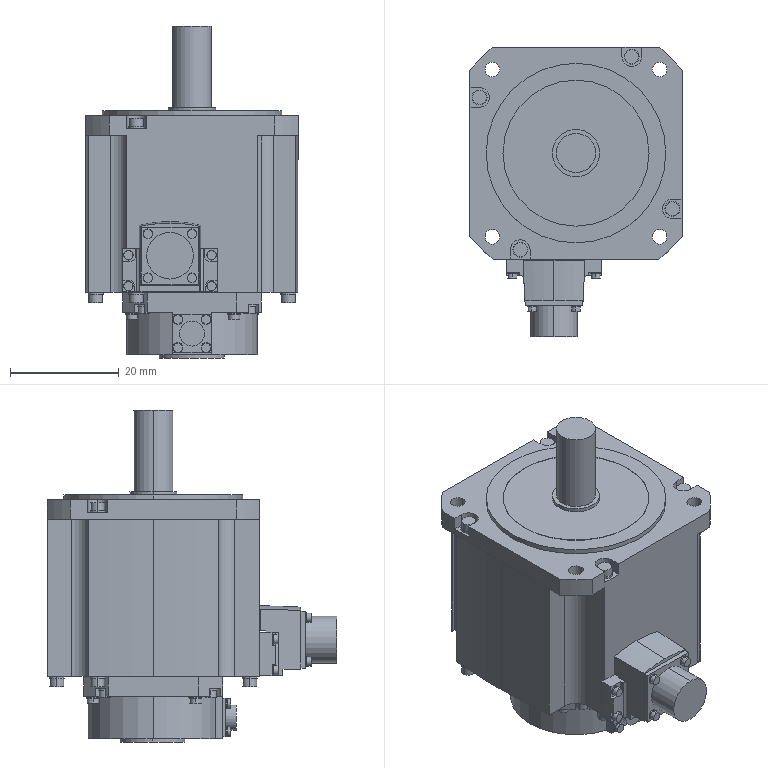Part | SolidWorks | features ICE 2, BaseBody 1, Scale 1 | 1 solid | 1997 faces | box 39 x 53.247 x 61.05 mm | volume 51590 mm3 | plane 1296 | spline 510 | cylinder 189 | cone 2 | commonest cylinder face diameters 1.77 x24 1.65 x16 2.1 x16 2.28 x16 2.4 x16 2.55 x16